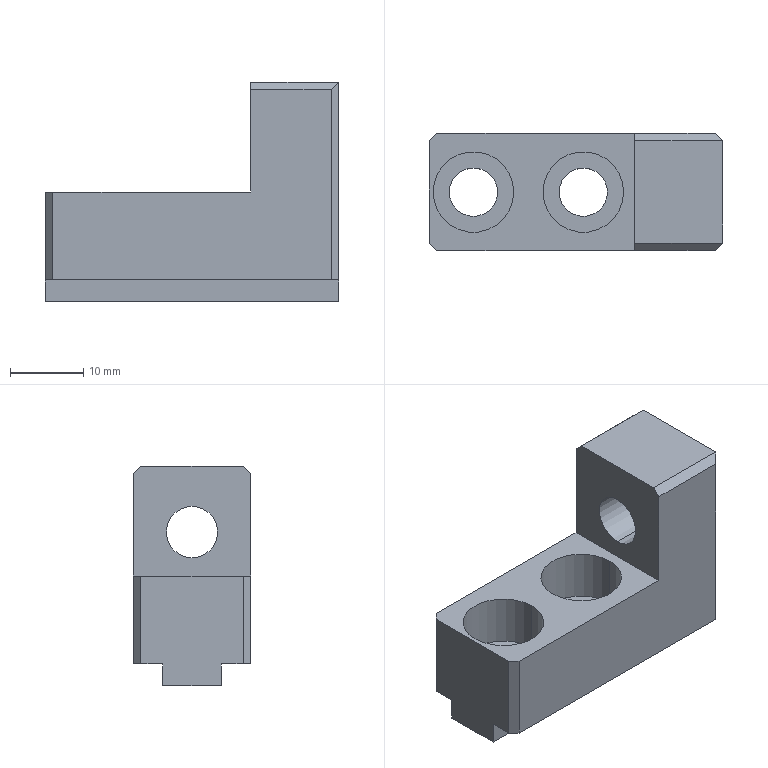Part | NX | features BREP 1 | 1 solid | 30 faces | box 40 x 16 x 30 mm | volume 9130 mm3 | plane 20 | cylinder 10 | commonest cylinder face diameters 6.6 x4 11 x4 7 x2
STEP:
#1=CARTESIAN_POINT('',(-4.5,0.,8.));
#2=VERTEX_POINT('',#1);
#3=CARTESIAN_POINT('',(6.5,0.,8.));
#4=VERTEX_POINT('',#3);
#5=CARTESIAN_POINT('',(1.,0.,8.));
#6=DIRECTION('',(0.,0.,1.));
#7=DIRECTION('',(1.,0.,0.));
#8=AXIS2_PLACEMENT_3D('',#5,#6,#7);
#9=CIRCLE('',#8,5.5);
#10=EDGE_CURVE('',#2,#4,#9,.T.);
#11=ORIENTED_EDGE('',*,*,#10,.F.);
#12=CARTESIAN_POINT('',(-4.5,0.,15.));
#13=VERTEX_POINT('',#12);
#14=CARTESIAN_POINT('',(-4.5,0.,15.));
#15=DIRECTION('',(0.,0.,1.));
#16=VECTOR('',#15,1000.);
#17=LINE('',#14,#16);
#18=EDGE_CURVE('',#13,#2,#17,.F.);
#19=ORIENTED_EDGE('',*,*,#18,.F.);
#20=CARTESIAN_POINT('',(6.5,0.,15.));
#21=VERTEX_POINT('',#20);
#22=CARTESIAN_POINT('',(1.,0.,15.));
#23=DIRECTION('',(0.,0.,1.));
#24=DIRECTION('',(1.,0.,0.));
#25=AXIS2_PLACEMENT_3D('',#22,#23,#24);
#26=CIRCLE('',#25,5.5);
#27=EDGE_CURVE('',#13,#21,#26,.T.);
#28=ORIENTED_EDGE('',*,*,#27,.T.);
#29=CARTESIAN_POINT('',(6.5,0.,15.));
#30=DIRECTION('',(0.,0.,1.));
#31=VECTOR('',#30,1000.);
#32=LINE('',#29,#31);
#33=EDGE_CURVE('',#21,#4,#32,.F.);
#34=ORIENTED_EDGE('',*,*,#33,.T.);
#35=EDGE_LOOP('',(#11,#19,#28,#34));
#36=FACE_BOUND('',#35,.T.);
#37=CARTESIAN_POINT('',(1.,0.,15.));
#38=DIRECTION('',(0.,0.,1.));
#39=DIRECTION('',(1.,0.,0.));
#40=AXIS2_PLACEMENT_3D('',#37,#38,#39);
#41=CYLINDRICAL_SURFACE('',#40,5.5);
#42=ADVANCED_FACE('',(#36),#41,.F.);
#43=CARTESIAN_POINT('',(-2.3,0.,0.));
#44=VERTEX_POINT('',#43);
#45=CARTESIAN_POINT('',(4.3,0.,0.));
#46=VERTEX_POINT('',#45);
#47=CARTESIAN_POINT('',(1.,0.,0.));
#48=DIRECTION('',(0.,0.,1.));
#49=DIRECTION('',(1.,0.,0.));
#50=AXIS2_PLACEMENT_3D('',#47,#48,#49);
#51=CIRCLE('',#50,3.3);
#52=EDGE_CURVE('',#44,#46,#51,.T.);
#53=ORIENTED_EDGE('',*,*,#52,.F.);
#54=CARTESIAN_POINT('',(-2.3,0.,8.));
#55=VERTEX_POINT('',#54);
#56=CARTESIAN_POINT('',(-2.3,0.,15.));
#57=DIRECTION('',(0.,0.,1.));
#58=VECTOR('',#57,1000.);
#59=LINE('',#56,#58);
#60=EDGE_CURVE('',#55,#44,#59,.F.);
#61=ORIENTED_EDGE('',*,*,#60,.F.);
#62=CARTESIAN_POINT('',(4.3,0.,8.));
#63=VERTEX_POINT('',#62);
#64=CARTESIAN_POINT('',(1.,0.,8.));
#65=DIRECTION('',(0.,0.,1.));
#66=DIRECTION('',(1.,0.,0.));
#67=AXIS2_PLACEMENT_3D('',#64,#65,#66);
#68=CIRCLE('',#67,3.3);
#69=EDGE_CURVE('',#55,#63,#68,.T.);
#70=ORIENTED_EDGE('',*,*,#69,.T.);
#71=CARTESIAN_POINT('',(4.3,0.,15.));
#72=DIRECTION('',(0.,0.,1.));
#73=VECTOR('',#72,1000.);
#74=LINE('',#71,#73);
#75=EDGE_CURVE('',#63,#46,#74,.F.);
#76=ORIENTED_EDGE('',*,*,#75,.T.);
#77=EDGE_LOOP('',(#53,#61,#70,#76));
#78=FACE_BOUND('',#77,.T.);
#79=CARTESIAN_POINT('',(1.,0.,15.));
#80=DIRECTION('',(0.,0.,1.));
#81=DIRECTION('',(1.,0.,0.));
#82=AXIS2_PLACEMENT_3D('',#79,#80,#81);
#83=CYLINDRICAL_SURFACE('',#82,3.3);
#84=ADVANCED_FACE('',(#78),#83,.F.);
#85=CARTESIAN_POINT('',(20.,0.,17.5));
#86=VERTEX_POINT('',#85);
#87=CARTESIAN_POINT('',(20.,0.,24.5));
#88=VERTEX_POINT('',#87);
#89=CARTESIAN_POINT('',(20.,0.,21.));
#90=DIRECTION('',(-1.,0.,0.));
#91=DIRECTION('',(0.,0.,1.));
#92=AXIS2_PLACEMENT_3D('',#89,#90,#91);
#93=CIRCLE('',#92,3.5);
#94=EDGE_CURVE('',#86,#88,#93,.T.);
#95=ORIENTED_EDGE('',*,*,#94,.F.);
#96=CARTESIAN_POINT('',(8.,0.,17.5));
#97=VERTEX_POINT('',#96);
#98=CARTESIAN_POINT('',(8.,0.,17.5));
#99=DIRECTION('',(-1.,0.,0.));
#100=VECTOR('',#99,1000.);
#101=LINE('',#98,#100);
#102=EDGE_CURVE('',#97,#86,#101,.F.);
#103=ORIENTED_EDGE('',*,*,#102,.F.);
#104=CARTESIAN_POINT('',(8.,0.,24.5));
#105=VERTEX_POINT('',#104);
#106=CARTESIAN_POINT('',(8.,0.,21.));
#107=DIRECTION('',(-1.,0.,0.));
#108=DIRECTION('',(0.,0.,1.));
#109=AXIS2_PLACEMENT_3D('',#106,#107,#108);
#110=CIRCLE('',#109,3.5);
#111=EDGE_CURVE('',#97,#105,#110,.T.);
#112=ORIENTED_EDGE('',*,*,#111,.T.);
#113=CARTESIAN_POINT('',(8.,0.,24.5));
#114=DIRECTION('',(-1.,0.,0.));
#115=VECTOR('',#114,1000.);
#116=LINE('',#113,#115);
#117=EDGE_CURVE('',#105,#88,#116,.F.);
#118=ORIENTED_EDGE('',*,*,#117,.T.);
#119=EDGE_LOOP('',(#95,#103,#112,#118));
#120=FACE_BOUND('',#119,.T.);
#121=CARTESIAN_POINT('',(8.,0.,21.));
#122=DIRECTION('',(-1.,0.,0.));
#123=DIRECTION('',(0.,0.,1.));
#124=AXIS2_PLACEMENT_3D('',#121,#122,#123);
#125=CYLINDRICAL_SURFACE('',#124,3.5);
#126=ADVANCED_FACE('',(#120),#125,.F.);
#127=CARTESIAN_POINT('',(-19.5,0.,8.));
#128=VERTEX_POINT('',#127);
#129=CARTESIAN_POINT('',(-8.5,0.,8.));
#130=VERTEX_POINT('',#129);
#131=CARTESIAN_POINT('',(-14.,0.,8.));
#132=DIRECTION('',(0.,0.,1.));
#133=DIRECTION('',(1.,0.,0.));
#134=AXIS2_PLACEMENT_3D('',#131,#132,#133);
#135=CIRCLE('',#134,5.5);
#136=EDGE_CURVE('',#128,#130,#135,.T.);
#137=ORIENTED_EDGE('',*,*,#136,.F.);
#138=CARTESIAN_POINT('',(-19.5,0.,15.));
#139=VERTEX_POINT('',#138);
#140=CARTESIAN_POINT('',(-19.5,0.,15.));
#141=DIRECTION('',(0.,0.,1.));
#142=VECTOR('',#141,1000.);
#143=LINE('',#140,#142);
#144=EDGE_CURVE('',#139,#128,#143,.F.);
#145=ORIENTED_EDGE('',*,*,#144,.F.);
#146=CARTESIAN_POINT('',(-8.5,0.,15.));
#147=VERTEX_POINT('',#146);
#148=CARTESIAN_POINT('',(-14.,0.,15.));
#149=DIRECTION('',(0.,0.,1.));
#150=DIRECTION('',(1.,0.,0.));
#151=AXIS2_PLACEMENT_3D('',#148,#149,#150);
#152=CIRCLE('',#151,5.5);
#153=EDGE_CURVE('',#139,#147,#152,.T.);
#154=ORIENTED_EDGE('',*,*,#153,.T.);
#155=CARTESIAN_POINT('',(-8.5,0.,15.));
#156=DIRECTION('',(0.,0.,1.));
#157=VECTOR('',#156,1000.);
#158=LINE('',#155,#157);
#159=EDGE_CURVE('',#147,#130,#158,.F.);
#160=ORIENTED_EDGE('',*,*,#159,.T.);
#161=EDGE_LOOP('',(#137,#145,#154,#160));
#162=FACE_BOUND('',#161,.T.);
#163=CARTESIAN_POINT('',(-14.,0.,15.));
#164=DIRECTION('',(0.,0.,1.));
#165=DIRECTION('',(1.,0.,0.));
#166=AXIS2_PLACEMENT_3D('',#163,#164,#165);
#167=CYLINDRICAL_SURFACE('',#166,5.5);
#168=ADVANCED_FACE('',(#162),#167,.F.);
#169=CARTESIAN_POINT('',(-17.3,0.,0.));
#170=VERTEX_POINT('',#169);
#171=CARTESIAN_POINT('',(-10.7,0.,0.));
#172=VERTEX_POINT('',#171);
#173=CARTESIAN_POINT('',(-14.,0.,0.));
#174=DIRECTION('',(0.,0.,1.));
#175=DIRECTION('',(1.,0.,0.));
#176=AXIS2_PLACEMENT_3D('',#173,#174,#175);
#177=CIRCLE('',#176,3.3);
#178=EDGE_CURVE('',#170,#172,#177,.T.);
#179=ORIENTED_EDGE('',*,*,#178,.F.);
#180=CARTESIAN_POINT('',(-17.3,0.,8.));
#181=VERTEX_POINT('',#180);
#182=CARTESIAN_POINT('',(-17.3,0.,15.));
#183=DIRECTION('',(0.,0.,1.));
#184=VECTOR('',#183,1000.);
#185=LINE('',#182,#184);
#186=EDGE_CURVE('',#181,#170,#185,.F.);
#187=ORIENTED_EDGE('',*,*,#186,.F.);
#188=CARTESIAN_POINT('',(-10.7,0.,8.));
#189=VERTEX_POINT('',#188);
#190=CARTESIAN_POINT('',(-14.,0.,8.));
#191=DIRECTION('',(0.,0.,1.));
#192=DIRECTION('',(1.,0.,0.));
#193=AXIS2_PLACEMENT_3D('',#190,#191,#192);
#194=CIRCLE('',#193,3.3);
#195=EDGE_CURVE('',#181,#189,#194,.T.);
#196=ORIENTED_EDGE('',*,*,#195,.T.);
#197=CARTESIAN_POINT('',(-10.7,0.,15.));
#198=DIRECTION('',(0.,0.,1.));
#199=VECTOR('',#198,1000.);
#200=LINE('',#197,#199);
#201=EDGE_CURVE('',#189,#172,#200,.F.);
#202=ORIENTED_EDGE('',*,*,#201,.T.);
#203=EDGE_LOOP('',(#179,#187,#196,#202));
#204=FACE_BOUND('',#203,.T.);
#205=CARTESIAN_POINT('',(-14.,0.,15.));
#206=DIRECTION('',(0.,0.,1.));
#207=DIRECTION('',(1.,0.,0.));
#208=AXIS2_PLACEMENT_3D('',#205,#206,#207);
#209=CYLINDRICAL_SURFACE('',#208,3.3);
#210=ADVANCED_FACE('',(#204),#209,.F.);
#211=CARTESIAN_POINT('',(-20.,-7.,3.));
#212=VERTEX_POINT('',#211);
#213=CARTESIAN_POINT('',(-20.,-4.,3.));
#214=VERTEX_POINT('',#213);
#215=CARTESIAN_POINT('',(-20.,-16.393,3.));
#216=DIRECTION('',(0.,1.,0.));
#217=VECTOR('',#216,1000.);
#218=LINE('',#215,#217);
#219=EDGE_CURVE('',#212,#214,#218,.T.);
#220=ORIENTED_EDGE('',*,*,#219,.F.);
#221=CARTESIAN_POINT('',(-20.,-7.,15.));
#222=VERTEX_POINT('',#221);
#223=CARTESIAN_POINT('',(-20.,-7.,30.));
#224=DIRECTION('',(0.,0.,1.));
#225=VECTOR('',#224,1000.);
#226=LINE('',#223,#225);
#227=EDGE_CURVE('',#212,#222,#226,.T.);
#228=ORIENTED_EDGE('',*,*,#227,.T.);
#229=CARTESIAN_POINT('',(-20.,7.,15.));
#230=VERTEX_POINT('',#229);
#231=CARTESIAN_POINT('',(-20.,-8.,15.));
#232=DIRECTION('',(0.,-1.,0.));
#233=VECTOR('',#232,1000.);
#234=LINE('',#231,#233);
#235=EDGE_CURVE('',#230,#222,#234,.T.);
#236=ORIENTED_EDGE('',*,*,#235,.F.);
#237=CARTESIAN_POINT('',(-20.,7.,3.));
#238=VERTEX_POINT('',#237);
#239=CARTESIAN_POINT('',(-20.,7.,30.));
#240=DIRECTION('',(0.,0.,-1.));
#241=VECTOR('',#240,1000.);
#242=LINE('',#239,#241);
#243=EDGE_CURVE('',#230,#238,#242,.T.);
#244=ORIENTED_EDGE('',*,*,#243,.T.);
#245=CARTESIAN_POINT('',(-20.,4.,3.));
#246=VERTEX_POINT('',#245);
#247=CARTESIAN_POINT('',(-20.,16.393,3.));
#248=DIRECTION('',(0.,1.,0.));
#249=VECTOR('',#248,1000.);
#250=LINE('',#247,#249);
#251=EDGE_CURVE('',#246,#238,#250,.T.);
#252=ORIENTED_EDGE('',*,*,#251,.F.);
#253=CARTESIAN_POINT('',(-20.,4.,0.));
#254=VERTEX_POINT('',#253);
#255=CARTESIAN_POINT('',(-20.,4.,-4.67));
#256=DIRECTION('',(0.,0.,1.));
#257=VECTOR('',#256,1000.);
#258=LINE('',#255,#257);
#259=EDGE_CURVE('',#254,#246,#258,.T.);
#260=ORIENTED_EDGE('',*,*,#259,.F.);
#261=CARTESIAN_POINT('',(-20.,-4.,0.));
#262=VERTEX_POINT('',#261);
#263=CARTESIAN_POINT('',(-20.,-8.,0.));
#264=DIRECTION('',(0.,-1.,0.));
#265=VECTOR('',#264,1000.);
#266=LINE('',#263,#265);
#267=EDGE_CURVE('',#254,#262,#266,.T.);
#268=ORIENTED_EDGE('',*,*,#267,.T.);
#269=CARTESIAN_POINT('',(-20.,-4.,-4.67));
#270=DIRECTION('',(0.,0.,-1.));
#271=VECTOR('',#270,1000.);
#272=LINE('',#269,#271);
#273=EDGE_CURVE('',#214,#262,#272,.T.);
#274=ORIENTED_EDGE('',*,*,#273,.F.);
#275=EDGE_LOOP('',(#220,#228,#236,#244,#252,#260,#268,#274));
#276=FACE_BOUND('',#275,.T.);
#277=CARTESIAN_POINT('',(-20.,-8.,30.));
#278=DIRECTION('',(1.,0.,0.));
#279=DIRECTION('',(0.,1.,0.));
#280=AXIS2_PLACEMENT_3D('',#277,#278,#279);
#281=PLANE('',#280);
#282=ADVANCED_FACE('',(#276),#281,.F.);
#283=CARTESIAN_POINT('',(19.,-8.,3.));
#284=VERTEX_POINT('',#283);
#285=CARTESIAN_POINT('',(19.,-8.,29.));
#286=VERTEX_POINT('',#285);
#287=CARTESIAN_POINT('',(19.,-8.,30.));
#288=DIRECTION('',(0.,0.,1.));
#289=VECTOR('',#288,1000.);
#290=LINE('',#287,#289);
#291=EDGE_CURVE('',#284,#286,#290,.T.);
#292=ORIENTED_EDGE('',*,*,#291,.T.);
#293=CARTESIAN_POINT('',(8.,-8.,29.));
#294=VERTEX_POINT('',#293);
#295=CARTESIAN_POINT('',(8.,-8.,29.));
#296=DIRECTION('',(-1.,0.,0.));
#297=VECTOR('',#296,1000.);
#298=LINE('',#295,#297);
#299=EDGE_CURVE('',#286,#294,#298,.T.);
#300=ORIENTED_EDGE('',*,*,#299,.T.);
#301=CARTESIAN_POINT('',(8.,-8.,15.));
#302=VERTEX_POINT('',#301);
#303=CARTESIAN_POINT('',(8.,-8.,30.));
#304=DIRECTION('',(0.,0.,-1.));
#305=VECTOR('',#304,1000.);
#306=LINE('',#303,#305);
#307=EDGE_CURVE('',#294,#302,#306,.T.);
#308=ORIENTED_EDGE('',*,*,#307,.T.);
#309=CARTESIAN_POINT('',(-19.,-8.,15.));
#310=VERTEX_POINT('',#309);
#311=CARTESIAN_POINT('',(20.,-8.,15.));
#312=DIRECTION('',(1.,0.,0.));
#313=VECTOR('',#312,1000.);
#314=LINE('',#311,#313);
#315=EDGE_CURVE('',#310,#302,#314,.T.);
#316=ORIENTED_EDGE('',*,*,#315,.F.);
#317=CARTESIAN_POINT('',(-19.,-8.,3.));
#318=VERTEX_POINT('',#317);
#319=CARTESIAN_POINT('',(-19.,-8.,30.));
#320=DIRECTION('',(0.,0.,-1.));
#321=VECTOR('',#320,1000.);
#322=LINE('',#319,#321);
#323=EDGE_CURVE('',#310,#318,#322,.T.);
#324=ORIENTED_EDGE('',*,*,#323,.T.);
#325=CARTESIAN_POINT('',(20.,-8.,3.));
#326=DIRECTION('',(1.,0.,0.));
#327=VECTOR('',#326,1000.);
#328=LINE('',#325,#327);
#329=EDGE_CURVE('',#318,#284,#328,.T.);
#330=ORIENTED_EDGE('',*,*,#329,.T.);
#331=EDGE_LOOP('',(#292,#300,#308,#316,#324,#330));
#332=FACE_BOUND('',#331,.T.);
#333=CARTESIAN_POINT('',(20.,-8.,30.));
#334=DIRECTION('',(0.,1.,0.));
#335=DIRECTION('',(1.,0.,0.));
#336=AXIS2_PLACEMENT_3D('',#333,#334,#335);
#337=PLANE('',#336);
#338=ADVANCED_FACE('',(#332),#337,.F.);
#339=CARTESIAN_POINT('',(20.,4.,3.));
#340=VERTEX_POINT('',#339);
#341=CARTESIAN_POINT('',(20.,7.,3.));
#342=VERTEX_POINT('',#341);
#343=CARTESIAN_POINT('',(20.,-8.,3.));
#344=DIRECTION('',(0.,1.,0.));
#345=VECTOR('',#344,1000.);
#346=LINE('',#343,#345);
#347=EDGE_CURVE('',#340,#342,#346,.T.);
#348=ORIENTED_EDGE('',*,*,#347,.T.);
#349=CARTESIAN_POINT('',(20.,7.,30.));
#350=VERTEX_POINT('',#349);
#351=CARTESIAN_POINT('',(20.,7.,30.));
#352=DIRECTION('',(0.,0.,1.));
#353=VECTOR('',#352,1000.);
#354=LINE('',#351,#353);
#355=EDGE_CURVE('',#342,#350,#354,.T.);
#356=ORIENTED_EDGE('',*,*,#355,.T.);
#357=CARTESIAN_POINT('',(20.,-7.,30.));
#358=VERTEX_POINT('',#357);
#359=CARTESIAN_POINT('',(20.,-8.,30.));
#360=DIRECTION('',(0.,1.,0.));
#361=VECTOR('',#360,1000.);
#362=LINE('',#359,#361);
#363=EDGE_CURVE('',#358,#350,#362,.T.);
#364=ORIENTED_EDGE('',*,*,#363,.F.);
#365=CARTESIAN_POINT('',(20.,-7.,3.));
#366=VERTEX_POINT('',#365);
#367=CARTESIAN_POINT('',(20.,-7.,30.));
#368=DIRECTION('',(0.,0.,-1.));
#369=VECTOR('',#368,1000.);
#370=LINE('',#367,#369);
#371=EDGE_CURVE('',#358,#366,#370,.T.);
#372=ORIENTED_EDGE('',*,*,#371,.T.);
#373=CARTESIAN_POINT('',(20.,-4.,3.));
#374=VERTEX_POINT('',#373);
#375=CARTESIAN_POINT('',(20.,-8.,3.));
#376=DIRECTION('',(0.,1.,0.));
#377=VECTOR('',#376,1000.);
#378=LINE('',#375,#377);
#379=EDGE_CURVE('',#366,#374,#378,.T.);
#380=ORIENTED_EDGE('',*,*,#379,.T.);
#381=CARTESIAN_POINT('',(20.,-4.,0.));
#382=VERTEX_POINT('',#381);
#383=CARTESIAN_POINT('',(20.,-4.,30.));
#384=DIRECTION('',(0.,0.,-1.));
#385=VECTOR('',#384,1000.);
#386=LINE('',#383,#385);
#387=EDGE_CURVE('',#374,#382,#386,.T.);
#388=ORIENTED_EDGE('',*,*,#387,.T.);
#389=CARTESIAN_POINT('',(20.,4.,0.));
#390=VERTEX_POINT('',#389);
#391=CARTESIAN_POINT('',(20.,-8.,0.));
#392=DIRECTION('',(0.,1.,0.));
#393=VECTOR('',#392,1000.);
#394=LINE('',#391,#393);
#395=EDGE_CURVE('',#382,#390,#394,.T.);
#396=ORIENTED_EDGE('',*,*,#395,.T.);
#397=CARTESIAN_POINT('',(20.,4.,30.));
#398=DIRECTION('',(0.,0.,1.));
#399=VECTOR('',#398,1000.);
#400=LINE('',#397,#399);
#401=EDGE_CURVE('',#390,#340,#400,.T.);
#402=ORIENTED_EDGE('',*,*,#401,.T.);
#403=EDGE_LOOP('',(#348,#356,#364,#372,#380,#388,#396,#402));
#404=FACE_BOUND('',#403,.T.);
#405=CARTESIAN_POINT('',(20.,0.,21.));
#406=DIRECTION('',(-1.,0.,0.));
#407=DIRECTION('',(0.,0.,1.));
#408=AXIS2_PLACEMENT_3D('',#405,#406,#407);
#409=CIRCLE('',#408,3.5);
#410=EDGE_CURVE('',#88,#86,#409,.T.);
#411=ORIENTED_EDGE('',*,*,#410,.T.);
#412=ORIENTED_EDGE('',*,*,#94,.T.);
#413=EDGE_LOOP('',(#411,#412));
#414=FACE_BOUND('',#413,.T.);
#415=CARTESIAN_POINT('',(20.,-8.,30.));
#416=DIRECTION('',(-1.,0.,0.));
#417=DIRECTION('',(0.,0.,1.));
#418=AXIS2_PLACEMENT_3D('',#415,#416,#417);
#419=PLANE('',#418);
#420=ADVANCED_FACE('',(#404,#414),#419,.F.);
#421=CARTESIAN_POINT('',(8.,8.,15.));
#422=VERTEX_POINT('',#421);
#423=CARTESIAN_POINT('',(8.,8.,29.));
#424=VERTEX_POINT('',#423);
#425=CARTESIAN_POINT('',(8.,8.,30.));
#426=DIRECTION('',(0.,0.,1.));
#427=VECTOR('',#426,1000.);
#428=LINE('',#425,#427);
#429=EDGE_CURVE('',#422,#424,#428,.T.);
#430=ORIENTED_EDGE('',*,*,#429,.T.);
#431=CARTESIAN_POINT('',(19.,8.,29.));
#432=VERTEX_POINT('',#431);
#433=CARTESIAN_POINT('',(20.,8.,29.));
#434=DIRECTION('',(1.,0.,0.));
#435=VECTOR('',#434,1000.);
#436=LINE('',#433,#435);
#437=EDGE_CURVE('',#424,#432,#436,.T.);
#438=ORIENTED_EDGE('',*,*,#437,.T.);
#439=CARTESIAN_POINT('',(19.,8.,3.));
#440=VERTEX_POINT('',#439);
#441=CARTESIAN_POINT('',(19.,8.,30.));
#442=DIRECTION('',(0.,0.,-1.));
#443=VECTOR('',#442,1000.);
#444=LINE('',#441,#443);
#445=EDGE_CURVE('',#432,#440,#444,.T.);
#446=ORIENTED_EDGE('',*,*,#445,.T.);
#447=CARTESIAN_POINT('',(-19.,8.,3.));
#448=VERTEX_POINT('',#447);
#449=CARTESIAN_POINT('',(20.,8.,3.));
#450=DIRECTION('',(-1.,0.,0.));
#451=VECTOR('',#450,1000.);
#452=LINE('',#449,#451);
#453=EDGE_CURVE('',#440,#448,#452,.T.);
#454=ORIENTED_EDGE('',*,*,#453,.T.);
#455=CARTESIAN_POINT('',(-19.,8.,15.));
#456=VERTEX_POINT('',#455);
#457=CARTESIAN_POINT('',(-19.,8.,30.));
#458=DIRECTION('',(0.,0.,1.));
#459=VECTOR('',#458,1000.);
#460=LINE('',#457,#459);
#461=EDGE_CURVE('',#448,#456,#460,.T.);
#462=ORIENTED_EDGE('',*,*,#461,.T.);
#463=CARTESIAN_POINT('',(20.,8.,15.));
#464=DIRECTION('',(-1.,0.,0.));
#465=VECTOR('',#464,1000.);
#466=LINE('',#463,#465);
#467=EDGE_CURVE('',#422,#456,#466,.T.);
#468=ORIENTED_EDGE('',*,*,#467,.F.);
#469=EDGE_LOOP('',(#430,#438,#446,#454,#462,#468));
#470=FACE_BOUND('',#469,.T.);
#471=CARTESIAN_POINT('',(20.,8.,30.));
#472=DIRECTION('',(0.,-1.,0.));
#473=DIRECTION('',(0.,0.,-1.));
#474=AXIS2_PLACEMENT_3D('',#471,#472,#473);
#475=PLANE('',#474);
#476=ADVANCED_FACE('',(#470),#475,.F.);
#477=ORIENTED_EDGE('',*,*,#363,.T.);
#478=CARTESIAN_POINT('',(8.,7.,30.));
#479=VERTEX_POINT('',#478);
#480=CARTESIAN_POINT('',(8.,7.,30.));
#481=DIRECTION('',(-1.,0.,0.));
#482=VECTOR('',#481,1000.);
#483=LINE('',#480,#482);
#484=EDGE_CURVE('',#350,#479,#483,.T.);
#485=ORIENTED_EDGE('',*,*,#484,.T.);
#486=CARTESIAN_POINT('',(8.,-7.,30.));
#487=VERTEX_POINT('',#486);
#488=CARTESIAN_POINT('',(8.,0.,30.));
#489=DIRECTION('',(0.,1.,0.));
#490=VECTOR('',#489,1000.);
#491=LINE('',#488,#490);
#492=EDGE_CURVE('',#487,#479,#491,.T.);
#493=ORIENTED_EDGE('',*,*,#492,.F.);
#494=CARTESIAN_POINT('',(20.,-7.,30.));
#495=DIRECTION('',(1.,0.,0.));
#496=VECTOR('',#495,1000.);
#497=LINE('',#494,#496);
#498=EDGE_CURVE('',#487,#358,#497,.T.);
#499=ORIENTED_EDGE('',*,*,#498,.T.);
#500=EDGE_LOOP('',(#477,#485,#493,#499));
#501=FACE_BOUND('',#500,.T.);
#502=CARTESIAN_POINT('',(0.,0.,30.));
#503=DIRECTION('',(0.,0.,1.));
#504=DIRECTION('',(1.,0.,0.));
#505=AXIS2_PLACEMENT_3D('',#502,#503,#504);
#506=PLANE('',#505);
#507=ADVANCED_FACE('',(#501),#506,.T.);
#508=ORIENTED_EDGE('',*,*,#395,.F.);
#509=CARTESIAN_POINT('',(0.,-4.,0.));
#510=DIRECTION('',(-1.,0.,0.));
#511=VECTOR('',#510,1000.);
#512=LINE('',#509,#511);
#513=EDGE_CURVE('',#382,#262,#512,.T.);
#514=ORIENTED_EDGE('',*,*,#513,.T.);
#515=ORIENTED_EDGE('',*,*,#267,.F.);
#516=CARTESIAN_POINT('',(0.,4.,0.));
#517=DIRECTION('',(1.,0.,0.));
#518=VECTOR('',#517,1000.);
#519=LINE('',#516,#518);
#520=EDGE_CURVE('',#254,#390,#519,.T.);
#521=ORIENTED_EDGE('',*,*,#520,.T.);
#522=EDGE_LOOP('',(#508,#514,#515,#521));
#523=FACE_BOUND('',#522,.T.);
#524=CARTESIAN_POINT('',(1.,0.,0.));
#525=DIRECTION('',(0.,0.,1.));
#526=DIRECTION('',(1.,0.,0.));
#527=AXIS2_PLACEMENT_3D('',#524,#525,#526);
#528=CIRCLE('',#527,3.3);
#529=EDGE_CURVE('',#46,#44,#528,.T.);
#530=ORIENTED_EDGE('',*,*,#529,.T.);
#531=ORIENTED_EDGE('',*,*,#52,.T.);
#532=EDGE_LOOP('',(#530,#531));
#533=FACE_BOUND('',#532,.T.);
#534=CARTESIAN_POINT('',(-14.,0.,0.));
#535=DIRECTION('',(0.,0.,1.));
#536=DIRECTION('',(1.,0.,0.));
#537=AXIS2_PLACEMENT_3D('',#534,#535,#536);
#538=CIRCLE('',#537,3.3);
#539=EDGE_CURVE('',#172,#170,#538,.T.);
#540=ORIENTED_EDGE('',*,*,#539,.T.);
#541=ORIENTED_EDGE('',*,*,#178,.T.);
#542=EDGE_LOOP('',(#540,#541));
#543=FACE_BOUND('',#542,.T.);
#544=CARTESIAN_POINT('',(0.,0.,0.));
#545=DIRECTION('',(0.,0.,1.));
#546=DIRECTION('',(1.,0.,0.));
#547=AXIS2_PLACEMENT_3D('',#544,#545,#546);
#548=PLANE('',#547);
#549=ADVANCED_FACE('',(#523,#533,#543),#548,.F.);
#550=ORIENTED_EDGE('',*,*,#235,.T.);
#551=CARTESIAN_POINT('',(-13.5,-13.5,15.));
#552=DIRECTION('',(0.7071,-0.7071,0.));
#553=VECTOR('',#552,1000.);
#554=LINE('',#551,#553);
#555=EDGE_CURVE('',#222,#310,#554,.T.);
#556=ORIENTED_EDGE('',*,*,#555,.T.);
#557=ORIENTED_EDGE('',*,*,#315,.T.);
#558=CARTESIAN_POINT('',(8.,18.317,15.));
#559=DIRECTION('',(0.,1.,0.));
#560=VECTOR('',#559,1000.);
#561=LINE('',#558,#560);
#562=EDGE_CURVE('',#302,#422,#561,.T.);
#563=ORIENTED_EDGE('',*,*,#562,.T.);
#564=ORIENTED_EDGE('',*,*,#467,.T.);
#565=CARTESIAN_POINT('',(-13.5,13.5,15.));
#566=DIRECTION('',(-0.7071,-0.7071,0.));
#567=VECTOR('',#566,1000.);
#568=LINE('',#565,#567);
#569=EDGE_CURVE('',#456,#230,#568,.T.);
#570=ORIENTED_EDGE('',*,*,#569,.T.);
#571=EDGE_LOOP('',(#550,#556,#557,#563,#564,#570));
#572=FACE_BOUND('',#571,.T.);
#573=CARTESIAN_POINT('',(1.,0.,15.));
#574=DIRECTION('',(0.,0.,1.));
#575=DIRECTION('',(1.,0.,0.));
#576=AXIS2_PLACEMENT_3D('',#573,#574,#575);
#577=CIRCLE('',#576,5.5);
#578=EDGE_CURVE('',#21,#13,#577,.T.);
#579=ORIENTED_EDGE('',*,*,#578,.F.);
#580=ORIENTED_EDGE('',*,*,#27,.F.);
#581=EDGE_LOOP('',(#579,#580));
#582=FACE_BOUND('',#581,.T.);
#583=CARTESIAN_POINT('',(-14.,0.,15.));
#584=DIRECTION('',(0.,0.,1.));
#585=DIRECTION('',(1.,0.,0.));
#586=AXIS2_PLACEMENT_3D('',#583,#584,#585);
#587=CIRCLE('',#586,5.5);
#588=EDGE_CURVE('',#147,#139,#587,.T.);
#589=ORIENTED_EDGE('',*,*,#588,.F.);
#590=ORIENTED_EDGE('',*,*,#153,.F.);
#591=EDGE_LOOP('',(#589,#590));
#592=FACE_BOUND('',#591,.T.);
#593=CARTESIAN_POINT('',(0.,0.,15.));
#594=DIRECTION('',(0.,0.,1.));
#595=DIRECTION('',(1.,0.,0.));
#596=AXIS2_PLACEMENT_3D('',#593,#594,#595);
#597=PLANE('',#596);
#598=ADVANCED_FACE('',(#572,#582,#592),#597,.T.);
#599=ORIENTED_EDGE('',*,*,#492,.T.);
#600=CARTESIAN_POINT('',(8.,7.,30.));
#601=DIRECTION('',(0.,0.7071,-0.7071));
#602=VECTOR('',#601,1000.);
#603=LINE('',#600,#602);
#604=EDGE_CURVE('',#479,#424,#603,.T.);
#605=ORIENTED_EDGE('',*,*,#604,.T.);
#606=ORIENTED_EDGE('',*,*,#429,.F.);
#607=ORIENTED_EDGE('',*,*,#562,.F.);
#608=ORIENTED_EDGE('',*,*,#307,.F.);
#609=CARTESIAN_POINT('',(8.,-7.,30.));
#610=DIRECTION('',(0.,0.7071,0.7071));
#611=VECTOR('',#610,1000.);
#612=LINE('',#609,#611);
#613=EDGE_CURVE('',#294,#487,#612,.T.);
#614=ORIENTED_EDGE('',*,*,#613,.T.);
#615=EDGE_LOOP('',(#599,#605,#606,#607,#608,#614));
#616=FACE_BOUND('',#615,.T.);
#617=CARTESIAN_POINT('',(8.,0.,21.));
#618=DIRECTION('',(-1.,0.,0.));
#619=DIRECTION('',(0.,0.,1.));
#620=AXIS2_PLACEMENT_3D('',#617,#618,#619);
#621=CIRCLE('',#620,3.5);
#622=EDGE_CURVE('',#105,#97,#621,.T.);
#623=ORIENTED_EDGE('',*,*,#622,.F.);
#624=ORIENTED_EDGE('',*,*,#111,.F.);
#625=EDGE_LOOP('',(#623,#624));
#626=FACE_BOUND('',#625,.T.);
#627=CARTESIAN_POINT('',(8.,18.317,15.));
#628=DIRECTION('',(1.,0.,0.));
#629=DIRECTION('',(0.,1.,0.));
#630=AXIS2_PLACEMENT_3D('',#627,#628,#629);
#631=PLANE('',#630);
#632=ADVANCED_FACE('',(#616,#626),#631,.F.);
#633=ORIENTED_EDGE('',*,*,#186,.T.);
#634=ORIENTED_EDGE('',*,*,#539,.F.);
#635=ORIENTED_EDGE('',*,*,#201,.F.);
#636=CARTESIAN_POINT('',(-14.,0.,8.));
#637=DIRECTION('',(0.,0.,1.));
#638=DIRECTION('',(1.,0.,0.));
#639=AXIS2_PLACEMENT_3D('',#636,#637,#638);
#640=CIRCLE('',#639,3.3);
#641=EDGE_CURVE('',#189,#181,#640,.T.);
#642=ORIENTED_EDGE('',*,*,#641,.T.);
#643=EDGE_LOOP('',(#633,#634,#635,#642));
#644=FACE_BOUND('',#643,.T.);
#645=CARTESIAN_POINT('',(-14.,0.,15.));
#646=DIRECTION('',(0.,0.,1.));
#647=DIRECTION('',(1.,0.,0.));
#648=AXIS2_PLACEMENT_3D('',#645,#646,#647);
#649=CYLINDRICAL_SURFACE('',#648,3.3);
#650=ADVANCED_FACE('',(#644),#649,.F.);
#651=CARTESIAN_POINT('',(-14.,0.,8.));
#652=DIRECTION('',(0.,0.,1.));
#653=DIRECTION('',(1.,0.,0.));
#654=AXIS2_PLACEMENT_3D('',#651,#652,#653);
#655=CIRCLE('',#654,5.5);
#656=EDGE_CURVE('',#130,#128,#655,.T.);
#657=ORIENTED_EDGE('',*,*,#656,.T.);
#658=ORIENTED_EDGE('',*,*,#136,.T.);
#659=EDGE_LOOP('',(#657,#658));
#660=FACE_BOUND('',#659,.T.);
#661=ORIENTED_EDGE('',*,*,#641,.F.);
#662=ORIENTED_EDGE('',*,*,#195,.F.);
#663=EDGE_LOOP('',(#661,#662));
#664=FACE_BOUND('',#663,.T.);
#665=CARTESIAN_POINT('',(-10.7,0.,8.));
#666=DIRECTION('',(0.,0.,-1.));
#667=DIRECTION('',(0.,-1.,0.));
#668=AXIS2_PLACEMENT_3D('',#665,#666,#667);
#669=PLANE('',#668);
#670=ADVANCED_FACE('',(#660,#664),#669,.F.);
#671=ORIENTED_EDGE('',*,*,#144,.T.);
#672=ORIENTED_EDGE('',*,*,#656,.F.);
#673=ORIENTED_EDGE('',*,*,#159,.F.);
#674=ORIENTED_EDGE('',*,*,#588,.T.);
#675=EDGE_LOOP('',(#671,#672,#673,#674));
#676=FACE_BOUND('',#675,.T.);
#677=CARTESIAN_POINT('',(-14.,0.,15.));
#678=DIRECTION('',(0.,0.,1.));
#679=DIRECTION('',(1.,0.,0.));
#680=AXIS2_PLACEMENT_3D('',#677,#678,#679);
#681=CYLINDRICAL_SURFACE('',#680,5.5);
#682=ADVANCED_FACE('',(#676),#681,.F.);
#683=ORIENTED_EDGE('',*,*,#453,.F.);
#684=CARTESIAN_POINT('',(19.,8.,3.));
#685=DIRECTION('',(0.7071,-0.7071,0.));
#686=VECTOR('',#685,1000.);
#687=LINE('',#684,#686);
#688=EDGE_CURVE('',#440,#342,#687,.T.);
#689=ORIENTED_EDGE('',*,*,#688,.T.);
#690=ORIENTED_EDGE('',*,*,#347,.F.);
#691=CARTESIAN_POINT('',(27.,4.,3.));
#692=DIRECTION('',(-1.,0.,0.));
#693=VECTOR('',#692,1000.);
#694=LINE('',#691,#693);
#695=EDGE_CURVE('',#340,#246,#694,.T.);
#696=ORIENTED_EDGE('',*,*,#695,.T.);
#697=ORIENTED_EDGE('',*,*,#251,.T.);
#698=CARTESIAN_POINT('',(-20.,7.,3.));
#699=DIRECTION('',(0.7071,0.7071,0.));
#700=VECTOR('',#699,1000.);
#701=LINE('',#698,#700);
#702=EDGE_CURVE('',#238,#448,#701,.T.);
#703=ORIENTED_EDGE('',*,*,#702,.T.);
#704=EDGE_LOOP('',(#683,#689,#690,#696,#697,#703));
#705=FACE_BOUND('',#704,.T.);
#706=CARTESIAN_POINT('',(27.,16.393,3.));
#707=DIRECTION('',(0.,0.,1.));
#708=DIRECTION('',(0.,-1.,0.));
#709=AXIS2_PLACEMENT_3D('',#706,#707,#708);
#710=PLANE('',#709);
#711=ADVANCED_FACE('',(#705),#710,.F.);
#712=ORIENTED_EDGE('',*,*,#520,.F.);
#713=ORIENTED_EDGE('',*,*,#259,.T.);
#714=ORIENTED_EDGE('',*,*,#695,.F.);
#715=ORIENTED_EDGE('',*,*,#401,.F.);
#716=EDGE_LOOP('',(#712,#713,#714,#715));
#717=FACE_BOUND('',#716,.T.);
#718=CARTESIAN_POINT('',(27.,4.,-4.67));
#719=DIRECTION('',(0.,-1.,0.));
#720=DIRECTION('',(0.,0.,-1.));
#721=AXIS2_PLACEMENT_3D('',#718,#719,#720);
#722=PLANE('',#721);
#723=ADVANCED_FACE('',(#717),#722,.F.);
#724=ORIENTED_EDGE('',*,*,#379,.F.);
#725=CARTESIAN_POINT('',(20.,-7.,3.));
#726=DIRECTION('',(-0.7071,-0.7071,0.));
#727=VECTOR('',#726,1000.);
#728=LINE('',#725,#727);
#729=EDGE_CURVE('',#366,#284,#728,.T.);
#730=ORIENTED_EDGE('',*,*,#729,.T.);
#731=ORIENTED_EDGE('',*,*,#329,.F.);
#732=CARTESIAN_POINT('',(-19.,-8.,3.));
#733=DIRECTION('',(-0.7071,0.7071,0.));
#734=VECTOR('',#733,1000.);
#735=LINE('',#732,#734);
#736=EDGE_CURVE('',#318,#212,#735,.T.);
#737=ORIENTED_EDGE('',*,*,#736,.T.);
#738=ORIENTED_EDGE('',*,*,#219,.T.);
#739=CARTESIAN_POINT('',(27.,-4.,3.));
#740=DIRECTION('',(-1.,0.,0.));
#741=VECTOR('',#740,1000.);
#742=LINE('',#739,#741);
#743=EDGE_CURVE('',#374,#214,#742,.T.);
#744=ORIENTED_EDGE('',*,*,#743,.F.);
#745=EDGE_LOOP('',(#724,#730,#731,#737,#738,#744));
#746=FACE_BOUND('',#745,.T.);
#747=CARTESIAN_POINT('',(27.,-16.393,3.));
#748=DIRECTION('',(0.,0.,1.));
#749=DIRECTION('',(0.,-1.,0.));
#750=AXIS2_PLACEMENT_3D('',#747,#748,#749);
#751=PLANE('',#750);
#752=ADVANCED_FACE('',(#746),#751,.F.);
#753=ORIENTED_EDGE('',*,*,#743,.T.);
#754=ORIENTED_EDGE('',*,*,#273,.T.);
#755=ORIENTED_EDGE('',*,*,#513,.F.);
#756=ORIENTED_EDGE('',*,*,#387,.F.);
#757=EDGE_LOOP('',(#753,#754,#755,#756));
#758=FACE_BOUND('',#757,.T.);
#759=CARTESIAN_POINT('',(27.,-4.,-4.67));
#760=DIRECTION('',(0.,1.,0.));
#761=DIRECTION('',(1.,0.,0.));
#762=AXIS2_PLACEMENT_3D('',#759,#760,#761);
#763=PLANE('',#762);
#764=ADVANCED_FACE('',(#758),#763,.F.);
#765=ORIENTED_EDGE('',*,*,#102,.T.);
#766=ORIENTED_EDGE('',*,*,#410,.F.);
#767=ORIENTED_EDGE('',*,*,#117,.F.);
#768=ORIENTED_EDGE('',*,*,#622,.T.);
#769=EDGE_LOOP('',(#765,#766,#767,#768));
#770=FACE_BOUND('',#769,.T.);
#771=CARTESIAN_POINT('',(8.,0.,21.));
#772=DIRECTION('',(-1.,0.,0.));
#773=DIRECTION('',(0.,0.,1.));
#774=AXIS2_PLACEMENT_3D('',#771,#772,#773);
#775=CYLINDRICAL_SURFACE('',#774,3.5);
#776=ADVANCED_FACE('',(#770),#775,.F.);
#777=ORIENTED_EDGE('',*,*,#688,.F.);
#778=ORIENTED_EDGE('',*,*,#445,.F.);
#779=CARTESIAN_POINT('',(19.333,7.667,29.333));
#780=DIRECTION('',(-0.5774,0.5774,-0.5774));
#781=VECTOR('',#780,1000.);
#782=LINE('',#779,#781);
#783=EDGE_CURVE('',#350,#432,#782,.T.);
#784=ORIENTED_EDGE('',*,*,#783,.F.);
#785=ORIENTED_EDGE('',*,*,#355,.F.);
#786=EDGE_LOOP('',(#777,#778,#784,#785));
#787=FACE_BOUND('',#786,.T.);
#788=CARTESIAN_POINT('',(19.,8.,30.));
#789=DIRECTION('',(-0.7071,-0.7071,0.));
#790=DIRECTION('',(-0.7071,0.7071,0.));
#791=AXIS2_PLACEMENT_3D('',#788,#789,#790);
#792=PLANE('',#791);
#793=ADVANCED_FACE('',(#787),#792,.F.);
#794=ORIENTED_EDGE('',*,*,#783,.T.);
#795=ORIENTED_EDGE('',*,*,#437,.F.);
#796=ORIENTED_EDGE('',*,*,#604,.F.);
#797=ORIENTED_EDGE('',*,*,#484,.F.);
#798=EDGE_LOOP('',(#794,#795,#796,#797));
#799=FACE_BOUND('',#798,.T.);
#800=CARTESIAN_POINT('',(0.,7.,30.));
#801=DIRECTION('',(0.,0.7071,0.7071));
#802=DIRECTION('',(1.,0.,0.));
#803=AXIS2_PLACEMENT_3D('',#800,#801,#802);
#804=PLANE('',#803);
#805=ADVANCED_FACE('',(#799),#804,.T.);
#806=ORIENTED_EDGE('',*,*,#729,.F.);
#807=ORIENTED_EDGE('',*,*,#371,.F.);
#808=CARTESIAN_POINT('',(20.,-7.,30.));
#809=DIRECTION('',(0.5774,0.5774,0.5774));
#810=VECTOR('',#809,1000.);
#811=LINE('',#808,#810);
#812=EDGE_CURVE('',#286,#358,#811,.T.);
#813=ORIENTED_EDGE('',*,*,#812,.F.);
#814=ORIENTED_EDGE('',*,*,#291,.F.);
#815=EDGE_LOOP('',(#806,#807,#813,#814));
#816=FACE_BOUND('',#815,.T.);
#817=CARTESIAN_POINT('',(20.,-7.,30.));
#818=DIRECTION('',(-0.7071,0.7071,0.));
#819=DIRECTION('',(0.,0.,1.));
#820=AXIS2_PLACEMENT_3D('',#817,#818,#819);
#821=PLANE('',#820);
#822=ADVANCED_FACE('',(#816),#821,.F.);
#823=ORIENTED_EDGE('',*,*,#613,.F.);
#824=ORIENTED_EDGE('',*,*,#299,.F.);
#825=ORIENTED_EDGE('',*,*,#812,.T.);
#826=ORIENTED_EDGE('',*,*,#498,.F.);
#827=EDGE_LOOP('',(#823,#824,#825,#826));
#828=FACE_BOUND('',#827,.T.);
#829=CARTESIAN_POINT('',(0.,-7.,30.));
#830=DIRECTION('',(0.,-0.7071,0.7071));
#831=DIRECTION('',(-1.,0.,0.));
#832=AXIS2_PLACEMENT_3D('',#829,#830,#831);
#833=PLANE('',#832);
#834=ADVANCED_FACE('',(#828),#833,.T.);
#835=ORIENTED_EDGE('',*,*,#555,.F.);
#836=ORIENTED_EDGE('',*,*,#227,.F.);
#837=ORIENTED_EDGE('',*,*,#736,.F.);
#838=ORIENTED_EDGE('',*,*,#323,.F.);
#839=EDGE_LOOP('',(#835,#836,#837,#838));
#840=FACE_BOUND('',#839,.T.);
#841=CARTESIAN_POINT('',(-19.,-8.,30.));
#842=DIRECTION('',(0.7071,0.7071,0.));
#843=DIRECTION('',(0.,0.,-1.));
#844=AXIS2_PLACEMENT_3D('',#841,#842,#843);
#845=PLANE('',#844);
#846=ADVANCED_FACE('',(#840),#845,.F.);
#847=ORIENTED_EDGE('',*,*,#569,.F.);
#848=ORIENTED_EDGE('',*,*,#461,.F.);
#849=ORIENTED_EDGE('',*,*,#702,.F.);
#850=ORIENTED_EDGE('',*,*,#243,.F.);
#851=EDGE_LOOP('',(#847,#848,#849,#850));
#852=FACE_BOUND('',#851,.T.);
#853=CARTESIAN_POINT('',(-20.,7.,30.));
#854=DIRECTION('',(0.7071,-0.7071,0.));
#855=DIRECTION('',(0.,0.,-1.));
#856=AXIS2_PLACEMENT_3D('',#853,#854,#855);
#857=PLANE('',#856);
#858=ADVANCED_FACE('',(#852),#857,.F.);
#859=ORIENTED_EDGE('',*,*,#60,.T.);
#860=ORIENTED_EDGE('',*,*,#529,.F.);
#861=ORIENTED_EDGE('',*,*,#75,.F.);
#862=CARTESIAN_POINT('',(1.,0.,8.));
#863=DIRECTION('',(0.,0.,1.));
#864=DIRECTION('',(1.,0.,0.));
#865=AXIS2_PLACEMENT_3D('',#862,#863,#864);
#866=CIRCLE('',#865,3.3);
#867=EDGE_CURVE('',#63,#55,#866,.T.);
#868=ORIENTED_EDGE('',*,*,#867,.T.);
#869=EDGE_LOOP('',(#859,#860,#861,#868));
#870=FACE_BOUND('',#869,.T.);
#871=CARTESIAN_POINT('',(1.,0.,15.));
#872=DIRECTION('',(0.,0.,1.));
#873=DIRECTION('',(1.,0.,0.));
#874=AXIS2_PLACEMENT_3D('',#871,#872,#873);
#875=CYLINDRICAL_SURFACE('',#874,3.3);
#876=ADVANCED_FACE('',(#870),#875,.F.);
#877=CARTESIAN_POINT('',(1.,0.,8.));
#878=DIRECTION('',(0.,0.,1.));
#879=DIRECTION('',(1.,0.,0.));
#880=AXIS2_PLACEMENT_3D('',#877,#878,#879);
#881=CIRCLE('',#880,5.5);
#882=EDGE_CURVE('',#4,#2,#881,.T.);
#883=ORIENTED_EDGE('',*,*,#882,.T.);
#884=ORIENTED_EDGE('',*,*,#10,.T.);
#885=EDGE_LOOP('',(#883,#884));
#886=FACE_BOUND('',#885,.T.);
#887=ORIENTED_EDGE('',*,*,#867,.F.);
#888=ORIENTED_EDGE('',*,*,#69,.F.);
#889=EDGE_LOOP('',(#887,#888));
#890=FACE_BOUND('',#889,.T.);
#891=CARTESIAN_POINT('',(4.3,0.,8.));
#892=DIRECTION('',(0.,0.,-1.));
#893=DIRECTION('',(0.,-1.,0.));
#894=AXIS2_PLACEMENT_3D('',#891,#892,#893);
#895=PLANE('',#894);
#896=ADVANCED_FACE('',(#886,#890),#895,.F.);
#897=ORIENTED_EDGE('',*,*,#18,.T.);
#898=ORIENTED_EDGE('',*,*,#882,.F.);
#899=ORIENTED_EDGE('',*,*,#33,.F.);
#900=ORIENTED_EDGE('',*,*,#578,.T.);
#901=EDGE_LOOP('',(#897,#898,#899,#900));
#902=FACE_BOUND('',#901,.T.);
#903=CARTESIAN_POINT('',(1.,0.,15.));
#904=DIRECTION('',(0.,0.,1.));
#905=DIRECTION('',(1.,0.,0.));
#906=AXIS2_PLACEMENT_3D('',#903,#904,#905);
#907=CYLINDRICAL_SURFACE('',#906,5.5);
#908=ADVANCED_FACE('',(#902),#907,.F.);
#909=CLOSED_SHELL('',(#42,#84,#126,#168,#210,#282,#338,#420,#476,#507,#549,#598,#632,#650,#670,#682,#711,#723,#752,#764,#776,#793,#805,#822,#834,#846,#858,#876,#896,#908));
#910=MANIFOLD_SOLID_BREP('',#909);
#911=(LENGTH_UNIT()NAMED_UNIT(*)SI_UNIT(.MILLI.,.METRE.));
#912=UNCERTAINTY_MEASURE_WITH_UNIT(LENGTH_MEASURE(0.00001),#911,'','');
#913=(NAMED_UNIT(*)PLANE_ANGLE_UNIT()SI_UNIT($,.RADIAN.));
#914=(NAMED_UNIT(*)SI_UNIT($,.STERADIAN.)SOLID_ANGLE_UNIT());
#915=(GEOMETRIC_REPRESENTATION_CONTEXT(3)GLOBAL_UNCERTAINTY_ASSIGNED_CONTEXT((#912))GLOBAL_UNIT_ASSIGNED_CONTEXT((#911,#913,#914))REPRESENTATION_CONTEXT('',''));
#916=ADVANCED_BREP_SHAPE_REPRESENTATION('',(#910),#915);